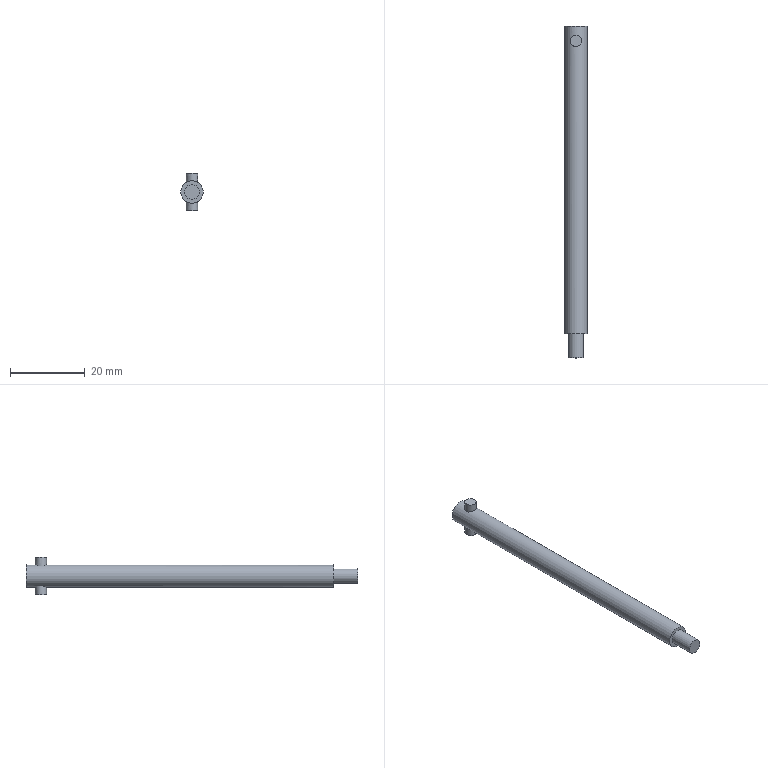Part | STEP file | 2-06.3 | 1 solid | 9 faces | box 6 x 89 x 10 mm | volume 2444 mm3 | plane 5 | cylinder 4 | commonest cylinder face diameters 3 x2 4 x1 6 x1
STEP:
#1=CARTESIAN_POINT('',(0.,0.,0.));
#2=DIRECTION('',(0.,0.,1.));
#3=DIRECTION('',(1.,0.,0.));
#4=AXIS2_PLACEMENT_3D('',#1,#2,#3);
#5=CARTESIAN_POINT('',(2.,-6.5,0.));
#6=VERTEX_POINT('',#5);
#7=CARTESIAN_POINT('',(0.,-6.5,0.));
#8=DIRECTION('',(0.,-1.,0.));
#9=DIRECTION('',(1.,0.,0.));
#10=AXIS2_PLACEMENT_3D('',#7,#8,#9);
#11=CIRCLE('',#10,2.);
#12=CARTESIAN_POINT('',(-0.5359,-6.5,0.));
#13=DIRECTION('',(0.,-1.,0.));
#14=DIRECTION('',(1.,0.,0.));
#15=AXIS2_PLACEMENT_3D('',#12,#13,#14);
#16=PLANE('',#15);
#17=CARTESIAN_POINT('',(0.5359,0.));
#18=DIRECTION('',(1.,0.));
#19=AXIS2_PLACEMENT_2D('',#17,#18);
#20=CIRCLE('',#19,2.);
#21=(GEOMETRIC_REPRESENTATION_CONTEXT(2)PARAMETRIC_REPRESENTATION_CONTEXT()REPRESENTATION_CONTEXT('',''));
#22=DEFINITIONAL_REPRESENTATION('',(#20),#21);
#23=PCURVE('',#16,#22);
#24=CARTESIAN_POINT('',(0.,0.,0.));
#25=DIRECTION('',(0.,-1.,0.));
#26=DIRECTION('',(1.,0.,0.));
#27=AXIS2_PLACEMENT_3D('',#24,#25,#26);
#28=CYLINDRICAL_SURFACE('',#27,2.);
#29=CARTESIAN_POINT('',(0.,6.5));
#30=DIRECTION('',(1.,0.));
#31=VECTOR('',#30,1.);
#32=LINE('',#29,#31);
#33=(GEOMETRIC_REPRESENTATION_CONTEXT(2)PARAMETRIC_REPRESENTATION_CONTEXT()REPRESENTATION_CONTEXT('',''));
#34=DEFINITIONAL_REPRESENTATION('',(#32),#33);
#35=PCURVE('',#28,#34);
#36=SURFACE_CURVE('',#11,(#23,#35),.PCURVE_S1.);
#37=EDGE_CURVE('',#6,#6,#36,.T.);
#38=ORIENTED_EDGE('',*,*,#37,.T.);
#39=EDGE_LOOP('',(#38));
#40=FACE_BOUND('',#39,.T.);
#41=ADVANCED_FACE('',(#40),#16,.T.);
#42=CARTESIAN_POINT('',(2.,0.,0.));
#43=VERTEX_POINT('',#42);
#44=CARTESIAN_POINT('',(0.,0.,0.));
#45=DIRECTION('',(0.,-1.,0.));
#46=DIRECTION('',(1.,0.,0.));
#47=AXIS2_PLACEMENT_3D('',#44,#45,#46);
#48=CIRCLE('',#47,2.);
#49=CARTESIAN_POINT('',(0.,0.));
#50=DIRECTION('',(1.,0.));
#51=VECTOR('',#50,1.);
#52=LINE('',#49,#51);
#53=(GEOMETRIC_REPRESENTATION_CONTEXT(2)PARAMETRIC_REPRESENTATION_CONTEXT()REPRESENTATION_CONTEXT('',''));
#54=DEFINITIONAL_REPRESENTATION('',(#52),#53);
#55=PCURVE('',#28,#54);
#56=CARTESIAN_POINT('',(-0.8038,0.,0.));
#57=DIRECTION('',(0.,-1.,0.));
#58=DIRECTION('',(1.,0.,0.));
#59=AXIS2_PLACEMENT_3D('',#56,#57,#58);
#60=PLANE('',#59);
#61=CARTESIAN_POINT('',(0.8038,0.));
#62=DIRECTION('',(1.,0.));
#63=AXIS2_PLACEMENT_2D('',#61,#62);
#64=CIRCLE('',#63,2.);
#65=(GEOMETRIC_REPRESENTATION_CONTEXT(2)PARAMETRIC_REPRESENTATION_CONTEXT()REPRESENTATION_CONTEXT('',''));
#66=DEFINITIONAL_REPRESENTATION('',(#64),#65);
#67=PCURVE('',#60,#66);
#68=SURFACE_CURVE('',#48,(#55,#67),.PCURVE_S1.);
#69=EDGE_CURVE('',#43,#43,#68,.T.);
#70=ORIENTED_EDGE('',*,*,#69,.T.);
#71=CARTESIAN_POINT('',(2.,0.,0.));
#72=DIRECTION('',(0.,-1.,0.));
#73=VECTOR('',#72,1.);
#74=LINE('',#71,#73);
#75=CARTESIAN_POINT('',(6.283,0.));
#76=DIRECTION('',(0.,1.));
#77=VECTOR('',#76,1.);
#78=LINE('',#75,#77);
#79=(GEOMETRIC_REPRESENTATION_CONTEXT(2)PARAMETRIC_REPRESENTATION_CONTEXT()REPRESENTATION_CONTEXT('',''));
#80=DEFINITIONAL_REPRESENTATION('',(#78),#79);
#81=PCURVE('',#28,#80);
#82=CARTESIAN_POINT('',(0.,0.));
#83=DIRECTION('',(0.,1.));
#84=VECTOR('',#83,1.);
#85=LINE('',#82,#84);
#86=(GEOMETRIC_REPRESENTATION_CONTEXT(2)PARAMETRIC_REPRESENTATION_CONTEXT()REPRESENTATION_CONTEXT('',''));
#87=DEFINITIONAL_REPRESENTATION('',(#85),#86);
#88=PCURVE('',#28,#87);
#89=SEAM_CURVE('',#74,(#81,#88),.PCURVE_S1.);
#90=EDGE_CURVE('',#43,#6,#89,.T.);
#91=ORIENTED_EDGE('',*,*,#90,.T.);
#92=ORIENTED_EDGE('',*,*,#37,.F.);
#93=ORIENTED_EDGE('',*,*,#90,.F.);
#94=EDGE_LOOP('',(#70,#91,#92,#93));
#95=FACE_BOUND('',#94,.T.);
#96=ADVANCED_FACE('',(#95),#28,.T.);
#97=CARTESIAN_POINT('',(3.,0.,0.));
#98=VERTEX_POINT('',#97);
#99=CARTESIAN_POINT('',(0.,0.,0.));
#100=DIRECTION('',(0.,-1.,0.));
#101=DIRECTION('',(1.,0.,0.));
#102=AXIS2_PLACEMENT_3D('',#99,#100,#101);
#103=CIRCLE('',#102,3.);
#104=CARTESIAN_POINT('',(0.8038,0.));
#105=DIRECTION('',(1.,0.));
#106=AXIS2_PLACEMENT_2D('',#104,#105);
#107=CIRCLE('',#106,3.);
#108=(GEOMETRIC_REPRESENTATION_CONTEXT(2)PARAMETRIC_REPRESENTATION_CONTEXT()REPRESENTATION_CONTEXT('',''));
#109=DEFINITIONAL_REPRESENTATION('',(#107),#108);
#110=PCURVE('',#60,#109);
#111=CARTESIAN_POINT('',(0.,0.,0.));
#112=DIRECTION('',(0.,1.,0.));
#113=DIRECTION('',(1.,0.,0.));
#114=AXIS2_PLACEMENT_3D('',#111,#112,#113);
#115=CYLINDRICAL_SURFACE('',#114,3.);
#116=CARTESIAN_POINT('',(6.283,0.));
#117=DIRECTION('',(-1.,0.));
#118=VECTOR('',#117,1.);
#119=LINE('',#116,#118);
#120=(GEOMETRIC_REPRESENTATION_CONTEXT(2)PARAMETRIC_REPRESENTATION_CONTEXT()REPRESENTATION_CONTEXT('',''));
#121=DEFINITIONAL_REPRESENTATION('',(#119),#120);
#122=PCURVE('',#115,#121);
#123=SURFACE_CURVE('',#103,(#110,#122),.PCURVE_S1.);
#124=EDGE_CURVE('',#98,#98,#123,.T.);
#125=ORIENTED_EDGE('',*,*,#124,.T.);
#126=EDGE_LOOP('',(#125));
#127=FACE_BOUND('',#126,.T.);
#128=ORIENTED_EDGE('',*,*,#69,.F.);
#129=EDGE_LOOP('',(#128));
#130=FACE_BOUND('',#129,.T.);
#131=ADVANCED_FACE('',(#127,#130),#60,.T.);
#132=CARTESIAN_POINT('',(3.,82.5,0.));
#133=VERTEX_POINT('',#132);
#134=CARTESIAN_POINT('',(3.,0.,0.));
#135=DIRECTION('',(0.,1.,0.));
#136=VECTOR('',#135,1.);
#137=LINE('',#134,#136);
#138=CARTESIAN_POINT('',(6.283,0.));
#139=DIRECTION('',(0.,1.));
#140=VECTOR('',#139,1.);
#141=LINE('',#138,#140);
#142=(GEOMETRIC_REPRESENTATION_CONTEXT(2)PARAMETRIC_REPRESENTATION_CONTEXT()REPRESENTATION_CONTEXT('',''));
#143=DEFINITIONAL_REPRESENTATION('',(#141),#142);
#144=PCURVE('',#115,#143);
#145=CARTESIAN_POINT('',(0.,0.));
#146=DIRECTION('',(0.,1.));
#147=VECTOR('',#146,1.);
#148=LINE('',#145,#147);
#149=(GEOMETRIC_REPRESENTATION_CONTEXT(2)PARAMETRIC_REPRESENTATION_CONTEXT()REPRESENTATION_CONTEXT('',''));
#150=DEFINITIONAL_REPRESENTATION('',(#148),#149);
#151=PCURVE('',#115,#150);
#152=SEAM_CURVE('',#137,(#144,#151),.PCURVE_S1.);
#153=EDGE_CURVE('',#98,#133,#152,.T.);
#154=ORIENTED_EDGE('',*,*,#153,.T.);
#155=CARTESIAN_POINT('',(0.,82.5,0.));
#156=DIRECTION('',(0.,-1.,0.));
#157=DIRECTION('',(1.,0.,0.));
#158=AXIS2_PLACEMENT_3D('',#155,#156,#157);
#159=CIRCLE('',#158,3.);
#160=CARTESIAN_POINT('',(6.283,82.5));
#161=DIRECTION('',(-1.,0.));
#162=VECTOR('',#161,1.);
#163=LINE('',#160,#162);
#164=(GEOMETRIC_REPRESENTATION_CONTEXT(2)PARAMETRIC_REPRESENTATION_CONTEXT()REPRESENTATION_CONTEXT('',''));
#165=DEFINITIONAL_REPRESENTATION('',(#163),#164);
#166=PCURVE('',#115,#165);
#167=CARTESIAN_POINT('',(-0.8038,82.5,0.));
#168=DIRECTION('',(0.,-1.,0.));
#169=DIRECTION('',(1.,0.,0.));
#170=AXIS2_PLACEMENT_3D('',#167,#168,#169);
#171=PLANE('',#170);
#172=CARTESIAN_POINT('',(0.8038,0.));
#173=DIRECTION('',(1.,0.));
#174=AXIS2_PLACEMENT_2D('',#172,#173);
#175=CIRCLE('',#174,3.);
#176=(GEOMETRIC_REPRESENTATION_CONTEXT(2)PARAMETRIC_REPRESENTATION_CONTEXT()REPRESENTATION_CONTEXT('',''));
#177=DEFINITIONAL_REPRESENTATION('',(#175),#176);
#178=PCURVE('',#171,#177);
#179=SURFACE_CURVE('',#159,(#166,#178),.PCURVE_S1.);
#180=EDGE_CURVE('',#133,#133,#179,.T.);
#181=ORIENTED_EDGE('',*,*,#180,.T.);
#182=ORIENTED_EDGE('',*,*,#153,.F.);
#183=ORIENTED_EDGE('',*,*,#124,.F.);
#184=EDGE_LOOP('',(#154,#181,#182,#183));
#185=FACE_BOUND('',#184,.T.);
#186=CARTESIAN_POINT('',(0.,80.,3.));
#187=VERTEX_POINT('',#186);
#188=CARTESIAN_POINT('',(0.,80.,3.));
#189=CARTESIAN_POINT('',(-0.2296,80.,3.));
#190=CARTESIAN_POINT('',(-0.9186,79.842,2.921));
#191=CARTESIAN_POINT('',(-1.37,79.258,2.671));
#192=CARTESIAN_POINT('',(-1.562,78.376,2.564));
#193=CARTESIAN_POINT('',(-1.456,77.934,2.639));
#194=CARTESIAN_POINT('',(-0.9093,77.221,2.875));
#195=CARTESIAN_POINT('',(-0.4758,77.,3.));
#196=CARTESIAN_POINT('',(0.5891,77.,3.));
#197=CARTESIAN_POINT('',(1.105,77.338,2.803));
#198=CARTESIAN_POINT('',(1.548,78.257,2.579));
#199=CARTESIAN_POINT('',(1.552,78.714,2.576));
#200=CARTESIAN_POINT('',(1.209,79.46,2.751));
#201=CARTESIAN_POINT('',(0.7747,79.887,2.944));
#202=CARTESIAN_POINT('',(0.1937,80.,3.));
#203=CARTESIAN_POINT('',(0.,80.,3.));
#204=B_SPLINE_CURVE_WITH_KNOTS('',3,(#188,#189,#190,#191,#192,#193,#194,#195,#196,#197,#198,#199,#200,#201,#202,#203),.UNSPECIFIED.,.T.,.F.,(1,3,1,2,2,2,2,2,1,3,1),(-0.2841,0.,0.3333,1.,1.674,2.382,3.26,3.963,4.531,4.815,5.148),.UNSPECIFIED.);
#205=CARTESIAN_POINT('',(4.712,80.));
#206=CARTESIAN_POINT('',(4.687,80.));
#207=CARTESIAN_POINT('',(4.637,79.989));
#208=CARTESIAN_POINT('',(4.563,79.939));
#209=CARTESIAN_POINT('',(4.492,79.857));
#210=CARTESIAN_POINT('',(4.426,79.744));
#211=CARTESIAN_POINT('',(4.365,79.605));
#212=CARTESIAN_POINT('',(4.311,79.442));
#213=CARTESIAN_POINT('',(4.265,79.26));
#214=CARTESIAN_POINT('',(4.228,79.061));
#215=CARTESIAN_POINT('',(4.202,78.85));
#216=CARTESIAN_POINT('',(4.189,78.633));
#217=CARTESIAN_POINT('',(4.188,78.419));
#218=CARTESIAN_POINT('',(4.198,78.21));
#219=CARTESIAN_POINT('',(4.219,78.008));
#220=CARTESIAN_POINT('',(4.249,77.815));
#221=CARTESIAN_POINT('',(4.29,77.635));
#222=CARTESIAN_POINT('',(4.339,77.469));
#223=CARTESIAN_POINT('',(4.393,77.325));
#224=CARTESIAN_POINT('',(4.453,77.206));
#225=CARTESIAN_POINT('',(4.518,77.111));
#226=CARTESIAN_POINT('',(4.585,77.043));
#227=CARTESIAN_POINT('',(4.656,77.004));
#228=CARTESIAN_POINT('',(4.729,76.996));
#229=CARTESIAN_POINT('',(4.801,77.018));
#230=CARTESIAN_POINT('',(4.87,77.07));
#231=CARTESIAN_POINT('',(4.936,77.149));
#232=CARTESIAN_POINT('',(4.998,77.254));
#233=CARTESIAN_POINT('',(5.055,77.381));
#234=CARTESIAN_POINT('',(5.106,77.531));
#235=CARTESIAN_POINT('',(5.151,77.699));
#236=CARTESIAN_POINT('',(5.188,77.887));
#237=CARTESIAN_POINT('',(5.215,78.083));
#238=CARTESIAN_POINT('',(5.232,78.283));
#239=CARTESIAN_POINT('',(5.238,78.486));
#240=CARTESIAN_POINT('',(5.233,78.689));
#241=CARTESIAN_POINT('',(5.218,78.89));
#242=CARTESIAN_POINT('',(5.192,79.087));
#243=CARTESIAN_POINT('',(5.156,79.277));
#244=CARTESIAN_POINT('',(5.11,79.453));
#245=CARTESIAN_POINT('',(5.056,79.611));
#246=CARTESIAN_POINT('',(4.996,79.748));
#247=CARTESIAN_POINT('',(4.93,79.859));
#248=CARTESIAN_POINT('',(4.86,79.94));
#249=CARTESIAN_POINT('',(4.787,79.989));
#250=CARTESIAN_POINT('',(4.737,80.));
#251=CARTESIAN_POINT('',(4.712,80.));
#252=B_SPLINE_CURVE_WITH_KNOTS('',3,(#205,#206,#207,#208,#209,#210,#211,#212,#213,#214,#215,#216,#217,#218,#219,#220,#221,#222,#223,#224,#225,#226,#227,#228,#229,#230,#231,#232,#233,#234,#235,#236,#237,#238,#239,#240,#241,#242,#243,#244,#245,#246,#247,#248,#249,#250,#251),.UNSPECIFIED.,.T.,.F.,(4,1,1,1,1,1,1,1,1,1,1,1,1,1,1,1,1,1,1,1,1,1,1,1,1,1,1,1,1,1,1,1,1,1,1,1,1,1,1,1,1,1,1,1,4),(0.,0.1094,0.2189,0.3283,0.4377,0.5472,0.6566,0.766,0.8755,0.9849,1.094,1.204,1.313,1.423,1.532,1.641,1.751,1.86,1.97,2.079,2.189,2.298,2.408,2.517,2.626,2.736,2.845,2.955,3.064,3.174,3.283,3.392,3.502,3.611,3.721,3.83,3.94,4.049,4.158,4.268,4.377,4.487,4.596,4.706,4.815),.QUASI_UNIFORM_KNOTS.);
#253=(GEOMETRIC_REPRESENTATION_CONTEXT(2)PARAMETRIC_REPRESENTATION_CONTEXT()REPRESENTATION_CONTEXT('',''));
#254=DEFINITIONAL_REPRESENTATION('',(#252),#253);
#255=PCURVE('',#115,#254);
#256=CARTESIAN_POINT('',(0.,78.5,5.));
#257=DIRECTION('',(0.,0.,-1.));
#258=DIRECTION('',(0.,1.,0.));
#259=AXIS2_PLACEMENT_3D('',#256,#257,#258);
#260=CYLINDRICAL_SURFACE('',#259,1.5);
#261=CARTESIAN_POINT('',(6.283,2.));
#262=CARTESIAN_POINT('',(6.233,2.));
#263=CARTESIAN_POINT('',(6.132,2.006));
#264=CARTESIAN_POINT('',(5.982,2.03));
#265=CARTESIAN_POINT('',(5.833,2.068));
#266=CARTESIAN_POINT('',(5.685,2.118));
#267=CARTESIAN_POINT('',(5.537,2.176));
#268=CARTESIAN_POINT('',(5.389,2.236));
#269=CARTESIAN_POINT('',(5.242,2.294));
#270=CARTESIAN_POINT('',(5.095,2.344));
#271=CARTESIAN_POINT('',(4.947,2.382));
#272=CARTESIAN_POINT('',(4.801,2.401));
#273=CARTESIAN_POINT('',(4.659,2.401));
#274=CARTESIAN_POINT('',(4.519,2.385));
#275=CARTESIAN_POINT('',(4.38,2.355));
#276=CARTESIAN_POINT('',(4.24,2.314));
#277=CARTESIAN_POINT('',(4.1,2.263));
#278=CARTESIAN_POINT('',(3.957,2.206));
#279=CARTESIAN_POINT('',(3.817,2.151));
#280=CARTESIAN_POINT('',(3.677,2.1));
#281=CARTESIAN_POINT('',(3.538,2.057));
#282=CARTESIAN_POINT('',(3.397,2.023));
#283=CARTESIAN_POINT('',(3.254,2.002));
#284=CARTESIAN_POINT('',(3.107,1.997));
#285=CARTESIAN_POINT('',(2.963,2.011));
#286=CARTESIAN_POINT('',(2.823,2.038));
#287=CARTESIAN_POINT('',(2.684,2.077));
#288=CARTESIAN_POINT('',(2.546,2.124));
#289=CARTESIAN_POINT('',(2.408,2.176));
#290=CARTESIAN_POINT('',(2.27,2.231));
#291=CARTESIAN_POINT('',(2.132,2.283));
#292=CARTESIAN_POINT('',(1.99,2.333));
#293=CARTESIAN_POINT('',(1.851,2.37));
#294=CARTESIAN_POINT('',(1.715,2.392));
#295=CARTESIAN_POINT('',(1.58,2.4));
#296=CARTESIAN_POINT('',(1.445,2.394));
#297=CARTESIAN_POINT('',(1.309,2.374));
#298=CARTESIAN_POINT('',(1.17,2.339));
#299=CARTESIAN_POINT('',(1.028,2.29));
#300=CARTESIAN_POINT('',(0.8841,2.234));
#301=CARTESIAN_POINT('',(0.7387,2.175));
#302=CARTESIAN_POINT('',(0.5924,2.118));
#303=CARTESIAN_POINT('',(0.4456,2.068));
#304=CARTESIAN_POINT('',(0.2979,2.029));
#305=CARTESIAN_POINT('',(0.1492,2.006));
#306=CARTESIAN_POINT('',(0.04975,2.));
#307=CARTESIAN_POINT('',(0.,2.));
#308=B_SPLINE_CURVE_WITH_KNOTS('',3,(#261,#262,#263,#264,#265,#266,#267,#268,#269,#270,#271,#272,#273,#274,#275,#276,#277,#278,#279,#280,#281,#282,#283,#284,#285,#286,#287,#288,#289,#290,#291,#292,#293,#294,#295,#296,#297,#298,#299,#300,#301,#302,#303,#304,#305,#306,#307),.UNSPECIFIED.,.F.,.F.,(4,1,1,1,1,1,1,1,1,1,1,1,1,1,1,1,1,1,1,1,1,1,1,1,1,1,1,1,1,1,1,1,1,1,1,1,1,1,1,1,1,1,1,1,4),(0.,0.1094,0.2189,0.3283,0.4377,0.5472,0.6566,0.766,0.8755,0.9849,1.094,1.204,1.313,1.423,1.532,1.641,1.751,1.86,1.97,2.079,2.189,2.298,2.408,2.517,2.626,2.736,2.845,2.955,3.064,3.174,3.283,3.392,3.502,3.611,3.721,3.83,3.94,4.049,4.158,4.268,4.377,4.487,4.596,4.706,4.815),.QUASI_UNIFORM_KNOTS.);
#309=(GEOMETRIC_REPRESENTATION_CONTEXT(2)PARAMETRIC_REPRESENTATION_CONTEXT()REPRESENTATION_CONTEXT('',''));
#310=DEFINITIONAL_REPRESENTATION('',(#308),#309);
#311=PCURVE('',#260,#310);
#312=SURFACE_CURVE('',#204,(#255,#311),.PCURVE_S1.);
#313=EDGE_CURVE('',#187,#187,#312,.T.);
#314=ORIENTED_EDGE('',*,*,#313,.F.);
#315=EDGE_LOOP('',(#314));
#316=FACE_BOUND('',#315,.T.);
#317=CARTESIAN_POINT('',(0.,80.,-3.));
#318=VERTEX_POINT('',#317);
#319=CARTESIAN_POINT('',(0.,80.,-3.));
#320=CARTESIAN_POINT('',(0.2297,80.,-3.));
#321=CARTESIAN_POINT('',(0.919,79.842,-2.921));
#322=CARTESIAN_POINT('',(1.37,79.258,-2.671));
#323=CARTESIAN_POINT('',(1.565,78.362,-2.562));
#324=CARTESIAN_POINT('',(1.45,77.906,-2.645));
#325=CARTESIAN_POINT('',(0.8584,77.177,-2.894));
#326=CARTESIAN_POINT('',(0.3873,76.966,-3.017));
#327=CARTESIAN_POINT('',(-0.6675,77.047,-2.977));
#328=CARTESIAN_POINT('',(-1.138,77.385,-2.787));
#329=CARTESIAN_POINT('',(-1.548,78.276,-2.578));
#330=CARTESIAN_POINT('',(-1.548,78.724,-2.578));
#331=CARTESIAN_POINT('',(-1.209,79.461,-2.751));
#332=CARTESIAN_POINT('',(-0.7742,79.888,-2.944));
#333=CARTESIAN_POINT('',(-0.1935,80.,-3.));
#334=CARTESIAN_POINT('',(0.,80.,-3.));
#335=B_SPLINE_CURVE_WITH_KNOTS('',3,(#319,#320,#321,#322,#323,#324,#325,#326,#327,#328,#329,#330,#331,#332,#333,#334),.UNSPECIFIED.,.T.,.F.,(1,3,1,2,2,2,2,2,1,3,1),(-0.2819,0.,0.3333,1.,1.696,2.446,3.271,3.951,4.515,4.797,5.13),.UNSPECIFIED.);
#336=CARTESIAN_POINT('',(1.571,80.));
#337=CARTESIAN_POINT('',(1.546,80.));
#338=CARTESIAN_POINT('',(1.496,79.989));
#339=CARTESIAN_POINT('',(1.422,79.939));
#340=CARTESIAN_POINT('',(1.351,79.858));
#341=CARTESIAN_POINT('',(1.285,79.746));
#342=CARTESIAN_POINT('',(1.225,79.608));
#343=CARTESIAN_POINT('',(1.171,79.446));
#344=CARTESIAN_POINT('',(1.125,79.265));
#345=CARTESIAN_POINT('',(1.088,79.067));
#346=CARTESIAN_POINT('',(1.062,78.858));
#347=CARTESIAN_POINT('',(1.048,78.641));
#348=CARTESIAN_POINT('',(1.046,78.429));
#349=CARTESIAN_POINT('',(1.056,78.22));
#350=CARTESIAN_POINT('',(1.076,78.019));
#351=CARTESIAN_POINT('',(1.106,77.827));
#352=CARTESIAN_POINT('',(1.145,77.647));
#353=CARTESIAN_POINT('',(1.193,77.481));
#354=CARTESIAN_POINT('',(1.247,77.336));
#355=CARTESIAN_POINT('',(1.306,77.215));
#356=CARTESIAN_POINT('',(1.369,77.119));
#357=CARTESIAN_POINT('',(1.436,77.049));
#358=CARTESIAN_POINT('',(1.505,77.007));
#359=CARTESIAN_POINT('',(1.577,76.995));
#360=CARTESIAN_POINT('',(1.65,77.014));
#361=CARTESIAN_POINT('',(1.72,77.063));
#362=CARTESIAN_POINT('',(1.787,77.139));
#363=CARTESIAN_POINT('',(1.85,77.242));
#364=CARTESIAN_POINT('',(1.908,77.368));
#365=CARTESIAN_POINT('',(1.96,77.516));
#366=CARTESIAN_POINT('',(2.006,77.684));
#367=CARTESIAN_POINT('',(2.044,77.871));
#368=CARTESIAN_POINT('',(2.072,78.069));
#369=CARTESIAN_POINT('',(2.089,78.271));
#370=CARTESIAN_POINT('',(2.096,78.475));
#371=CARTESIAN_POINT('',(2.092,78.679));
#372=CARTESIAN_POINT('',(2.077,78.882));
#373=CARTESIAN_POINT('',(2.052,79.081));
#374=CARTESIAN_POINT('',(2.016,79.272));
#375=CARTESIAN_POINT('',(1.97,79.45));
#376=CARTESIAN_POINT('',(1.916,79.609));
#377=CARTESIAN_POINT('',(1.855,79.746));
#378=CARTESIAN_POINT('',(1.789,79.858));
#379=CARTESIAN_POINT('',(1.719,79.939));
#380=CARTESIAN_POINT('',(1.646,79.989));
#381=CARTESIAN_POINT('',(1.596,80.));
#382=CARTESIAN_POINT('',(1.571,80.));
#383=B_SPLINE_CURVE_WITH_KNOTS('',3,(#336,#337,#338,#339,#340,#341,#342,#343,#344,#345,#346,#347,#348,#349,#350,#351,#352,#353,#354,#355,#356,#357,#358,#359,#360,#361,#362,#363,#364,#365,#366,#367,#368,#369,#370,#371,#372,#373,#374,#375,#376,#377,#378,#379,#380,#381,#382),.UNSPECIFIED.,.T.,.F.,(4,1,1,1,1,1,1,1,1,1,1,1,1,1,1,1,1,1,1,1,1,1,1,1,1,1,1,1,1,1,1,1,1,1,1,1,1,1,1,1,1,1,1,1,4),(0.,0.109,0.218,0.327,0.4361,0.5451,0.6541,0.7631,0.8721,0.9811,1.09,1.199,1.308,1.417,1.526,1.635,1.744,1.853,1.962,2.071,2.18,2.289,2.398,2.507,2.616,2.725,2.834,2.943,3.052,3.161,3.27,3.379,3.488,3.597,3.706,3.815,3.924,4.033,4.142,4.251,4.361,4.47,4.579,4.688,4.797),.QUASI_UNIFORM_KNOTS.);
#384=(GEOMETRIC_REPRESENTATION_CONTEXT(2)PARAMETRIC_REPRESENTATION_CONTEXT()REPRESENTATION_CONTEXT('',''));
#385=DEFINITIONAL_REPRESENTATION('',(#383),#384);
#386=PCURVE('',#115,#385);
#387=CARTESIAN_POINT('',(0.,78.5,5.));
#388=DIRECTION('',(0.,0.,-1.));
#389=DIRECTION('',(0.,1.,0.));
#390=AXIS2_PLACEMENT_3D('',#387,#388,#389);
#391=CYLINDRICAL_SURFACE('',#390,1.5);
#392=CARTESIAN_POINT('',(0.,8.));
#393=CARTESIAN_POINT('',(0.05009,8.));
#394=CARTESIAN_POINT('',(0.1503,7.994));
#395=CARTESIAN_POINT('',(0.3001,7.971));
#396=CARTESIAN_POINT('',(0.4489,7.933));
#397=CARTESIAN_POINT('',(0.5964,7.883));
#398=CARTESIAN_POINT('',(0.7435,7.825));
#399=CARTESIAN_POINT('',(0.8906,7.765));
#400=CARTESIAN_POINT('',(1.038,7.708));
#401=CARTESIAN_POINT('',(1.184,7.658));
#402=CARTESIAN_POINT('',(1.331,7.619));
#403=CARTESIAN_POINT('',(1.477,7.6));
#404=CARTESIAN_POINT('',(1.618,7.599));
#405=CARTESIAN_POINT('',(1.758,7.614));
#406=CARTESIAN_POINT('',(1.896,7.643));
#407=CARTESIAN_POINT('',(2.034,7.683));
#408=CARTESIAN_POINT('',(2.173,7.733));
#409=CARTESIAN_POINT('',(2.315,7.79));
#410=CARTESIAN_POINT('',(2.454,7.844));
#411=CARTESIAN_POINT('',(2.593,7.895));
#412=CARTESIAN_POINT('',(2.732,7.938));
#413=CARTESIAN_POINT('',(2.87,7.973));
#414=CARTESIAN_POINT('',(3.011,7.995));
#415=CARTESIAN_POINT('',(3.154,8.003));
#416=CARTESIAN_POINT('',(3.301,7.993));
#417=CARTESIAN_POINT('',(3.443,7.967));
#418=CARTESIAN_POINT('',(3.584,7.929));
#419=CARTESIAN_POINT('',(3.723,7.882));
#420=CARTESIAN_POINT('',(3.861,7.83));
#421=CARTESIAN_POINT('',(4.,7.775));
#422=CARTESIAN_POINT('',(4.139,7.721));
#423=CARTESIAN_POINT('',(4.281,7.671));
#424=CARTESIAN_POINT('',(4.422,7.632));
#425=CARTESIAN_POINT('',(4.56,7.608));
#426=CARTESIAN_POINT('',(4.696,7.599));
#427=CARTESIAN_POINT('',(4.832,7.605));
#428=CARTESIAN_POINT('',(4.969,7.625));
#429=CARTESIAN_POINT('',(5.108,7.66));
#430=CARTESIAN_POINT('',(5.251,7.709));
#431=CARTESIAN_POINT('',(5.396,7.765));
#432=CARTESIAN_POINT('',(5.542,7.824));
#433=CARTESIAN_POINT('',(5.689,7.881));
#434=CARTESIAN_POINT('',(5.836,7.932));
#435=CARTESIAN_POINT('',(5.984,7.97));
#436=CARTESIAN_POINT('',(6.133,7.994));
#437=CARTESIAN_POINT('',(6.233,8.));
#438=CARTESIAN_POINT('',(6.283,8.));
#439=B_SPLINE_CURVE_WITH_KNOTS('',3,(#392,#393,#394,#395,#396,#397,#398,#399,#400,#401,#402,#403,#404,#405,#406,#407,#408,#409,#410,#411,#412,#413,#414,#415,#416,#417,#418,#419,#420,#421,#422,#423,#424,#425,#426,#427,#428,#429,#430,#431,#432,#433,#434,#435,#436,#437,#438),.UNSPECIFIED.,.F.,.F.,(4,1,1,1,1,1,1,1,1,1,1,1,1,1,1,1,1,1,1,1,1,1,1,1,1,1,1,1,1,1,1,1,1,1,1,1,1,1,1,1,1,1,1,1,4),(0.,0.109,0.218,0.327,0.4361,0.5451,0.6541,0.7631,0.8721,0.9811,1.09,1.199,1.308,1.417,1.526,1.635,1.744,1.853,1.962,2.071,2.18,2.289,2.398,2.507,2.616,2.725,2.834,2.943,3.052,3.161,3.27,3.379,3.488,3.597,3.706,3.815,3.924,4.033,4.142,4.251,4.361,4.47,4.579,4.688,4.797),.QUASI_UNIFORM_KNOTS.);
#440=(GEOMETRIC_REPRESENTATION_CONTEXT(2)PARAMETRIC_REPRESENTATION_CONTEXT()REPRESENTATION_CONTEXT('',''));
#441=DEFINITIONAL_REPRESENTATION('',(#439),#440);
#442=PCURVE('',#391,#441);
#443=SURFACE_CURVE('',#335,(#386,#442),.PCURVE_S1.);
#444=EDGE_CURVE('',#318,#318,#443,.T.);
#445=ORIENTED_EDGE('',*,*,#444,.F.);
#446=EDGE_LOOP('',(#445));
#447=FACE_BOUND('',#446,.T.);
#448=ADVANCED_FACE('',(#185,#316,#447),#115,.T.);
#449=CARTESIAN_POINT('',(0.,80.,-5.));
#450=VERTEX_POINT('',#449);
#451=CARTESIAN_POINT('',(0.,80.,-3.));
#452=DIRECTION('',(0.,0.,-1.));
#453=VECTOR('',#452,1.);
#454=LINE('',#451,#453);
#455=CARTESIAN_POINT('',(0.,8.));
#456=DIRECTION('',(0.,1.));
#457=VECTOR('',#456,1.);
#458=LINE('',#455,#457);
#459=(GEOMETRIC_REPRESENTATION_CONTEXT(2)PARAMETRIC_REPRESENTATION_CONTEXT()REPRESENTATION_CONTEXT('',''));
#460=DEFINITIONAL_REPRESENTATION('',(#458),#459);
#461=PCURVE('',#391,#460);
#462=CARTESIAN_POINT('',(6.283,8.));
#463=DIRECTION('',(0.,1.));
#464=VECTOR('',#463,1.);
#465=LINE('',#462,#464);
#466=(GEOMETRIC_REPRESENTATION_CONTEXT(2)PARAMETRIC_REPRESENTATION_CONTEXT()REPRESENTATION_CONTEXT('',''));
#467=DEFINITIONAL_REPRESENTATION('',(#465),#466);
#468=PCURVE('',#391,#467);
#469=SEAM_CURVE('',#454,(#461,#468),.PCURVE_S1.);
#470=EDGE_CURVE('',#318,#450,#469,.T.);
#471=ORIENTED_EDGE('',*,*,#470,.F.);
#472=ORIENTED_EDGE('',*,*,#444,.T.);
#473=ORIENTED_EDGE('',*,*,#470,.T.);
#474=CARTESIAN_POINT('',(0.,78.5,-5.));
#475=DIRECTION('',(0.,0.,1.));
#476=DIRECTION('',(0.,1.,0.));
#477=AXIS2_PLACEMENT_3D('',#474,#475,#476);
#478=CIRCLE('',#477,1.5);
#479=CARTESIAN_POINT('',(6.283,10.));
#480=DIRECTION('',(-1.,0.));
#481=VECTOR('',#480,1.);
#482=LINE('',#479,#481);
#483=(GEOMETRIC_REPRESENTATION_CONTEXT(2)PARAMETRIC_REPRESENTATION_CONTEXT()REPRESENTATION_CONTEXT('',''));
#484=DEFINITIONAL_REPRESENTATION('',(#482),#483);
#485=PCURVE('',#391,#484);
#486=CARTESIAN_POINT('',(0.,78.098,-5.));
#487=DIRECTION('',(0.,0.,1.));
#488=DIRECTION('',(0.,1.,0.));
#489=AXIS2_PLACEMENT_3D('',#486,#487,#488);
#490=PLANE('',#489);
#491=CARTESIAN_POINT('',(0.4019,0.));
#492=DIRECTION('',(1.,0.));
#493=AXIS2_PLACEMENT_2D('',#491,#492);
#494=CIRCLE('',#493,1.5);
#495=(GEOMETRIC_REPRESENTATION_CONTEXT(2)PARAMETRIC_REPRESENTATION_CONTEXT()REPRESENTATION_CONTEXT('',''));
#496=DEFINITIONAL_REPRESENTATION('',(#494),#495);
#497=PCURVE('',#490,#496);
#498=SURFACE_CURVE('',#478,(#485,#497),.PCURVE_S1.);
#499=EDGE_CURVE('',#450,#450,#498,.T.);
#500=ORIENTED_EDGE('',*,*,#499,.T.);
#501=EDGE_LOOP('',(#471,#472,#473,#500));
#502=FACE_BOUND('',#501,.T.);
#503=ADVANCED_FACE('',(#502),#391,.T.);
#504=ORIENTED_EDGE('',*,*,#499,.T.);
#505=EDGE_LOOP('',(#504));
#506=FACE_BOUND('',#505,.F.);
#507=ADVANCED_FACE('',(#506),#490,.F.);
#508=CARTESIAN_POINT('',(0.,80.,5.));
#509=VERTEX_POINT('',#508);
#510=CARTESIAN_POINT('',(0.,80.,5.));
#511=DIRECTION('',(0.,0.,-1.));
#512=VECTOR('',#511,1.);
#513=LINE('',#510,#512);
#514=CARTESIAN_POINT('',(6.283,0.));
#515=DIRECTION('',(0.,1.));
#516=VECTOR('',#515,1.);
#517=LINE('',#514,#516);
#518=(GEOMETRIC_REPRESENTATION_CONTEXT(2)PARAMETRIC_REPRESENTATION_CONTEXT()REPRESENTATION_CONTEXT('',''));
#519=DEFINITIONAL_REPRESENTATION('',(#517),#518);
#520=PCURVE('',#260,#519);
#521=CARTESIAN_POINT('',(0.,0.));
#522=DIRECTION('',(0.,1.));
#523=VECTOR('',#522,1.);
#524=LINE('',#521,#523);
#525=(GEOMETRIC_REPRESENTATION_CONTEXT(2)PARAMETRIC_REPRESENTATION_CONTEXT()REPRESENTATION_CONTEXT('',''));
#526=DEFINITIONAL_REPRESENTATION('',(#524),#525);
#527=PCURVE('',#260,#526);
#528=SEAM_CURVE('',#513,(#520,#527),.PCURVE_S1.);
#529=EDGE_CURVE('',#509,#187,#528,.T.);
#530=ORIENTED_EDGE('',*,*,#529,.T.);
#531=ORIENTED_EDGE('',*,*,#313,.T.);
#532=ORIENTED_EDGE('',*,*,#529,.F.);
#533=CARTESIAN_POINT('',(0.,78.5,5.));
#534=DIRECTION('',(0.,0.,1.));
#535=DIRECTION('',(0.,1.,0.));
#536=AXIS2_PLACEMENT_3D('',#533,#534,#535);
#537=CIRCLE('',#536,1.5);
#538=CARTESIAN_POINT('',(6.283,0.));
#539=DIRECTION('',(-1.,0.));
#540=VECTOR('',#539,1.);
#541=LINE('',#538,#540);
#542=(GEOMETRIC_REPRESENTATION_CONTEXT(2)PARAMETRIC_REPRESENTATION_CONTEXT()REPRESENTATION_CONTEXT('',''));
#543=DEFINITIONAL_REPRESENTATION('',(#541),#542);
#544=PCURVE('',#260,#543);
#545=CARTESIAN_POINT('',(0.,78.098,5.));
#546=DIRECTION('',(0.,0.,1.));
#547=DIRECTION('',(0.,1.,0.));
#548=AXIS2_PLACEMENT_3D('',#545,#546,#547);
#549=PLANE('',#548);
#550=CARTESIAN_POINT('',(0.4019,0.));
#551=DIRECTION('',(1.,0.));
#552=AXIS2_PLACEMENT_2D('',#550,#551);
#553=CIRCLE('',#552,1.5);
#554=(GEOMETRIC_REPRESENTATION_CONTEXT(2)PARAMETRIC_REPRESENTATION_CONTEXT()REPRESENTATION_CONTEXT('',''));
#555=DEFINITIONAL_REPRESENTATION('',(#553),#554);
#556=PCURVE('',#549,#555);
#557=SURFACE_CURVE('',#537,(#544,#556),.PCURVE_S1.);
#558=EDGE_CURVE('',#509,#509,#557,.T.);
#559=ORIENTED_EDGE('',*,*,#558,.F.);
#560=EDGE_LOOP('',(#530,#531,#532,#559));
#561=FACE_BOUND('',#560,.T.);
#562=ADVANCED_FACE('',(#561),#260,.T.);
#563=ORIENTED_EDGE('',*,*,#558,.T.);
#564=EDGE_LOOP('',(#563));
#565=FACE_BOUND('',#564,.T.);
#566=ADVANCED_FACE('',(#565),#549,.T.);
#567=ORIENTED_EDGE('',*,*,#180,.T.);
#568=EDGE_LOOP('',(#567));
#569=FACE_BOUND('',#568,.F.);
#570=ADVANCED_FACE('',(#569),#171,.F.);
#571=CLOSED_SHELL('',(#41,#96,#131,#448,#503,#507,#562,#566,#570));
#572=MANIFOLD_SOLID_BREP('',#571);
#573=(LENGTH_UNIT()NAMED_UNIT(*)SI_UNIT(.MILLI.,.METRE.));
#574=UNCERTAINTY_MEASURE_WITH_UNIT(LENGTH_MEASURE(0.001),#573,'','');
#575=(NAMED_UNIT(*)PLANE_ANGLE_UNIT()SI_UNIT($,.RADIAN.));
#576=(NAMED_UNIT(*)SI_UNIT($,.STERADIAN.)SOLID_ANGLE_UNIT());
#577=(GEOMETRIC_REPRESENTATION_CONTEXT(3)GLOBAL_UNCERTAINTY_ASSIGNED_CONTEXT((#574))GLOBAL_UNIT_ASSIGNED_CONTEXT((#573,#575,#576))REPRESENTATION_CONTEXT('',''));
#578=ADVANCED_BREP_SHAPE_REPRESENTATION('',(#4,#572),#577);